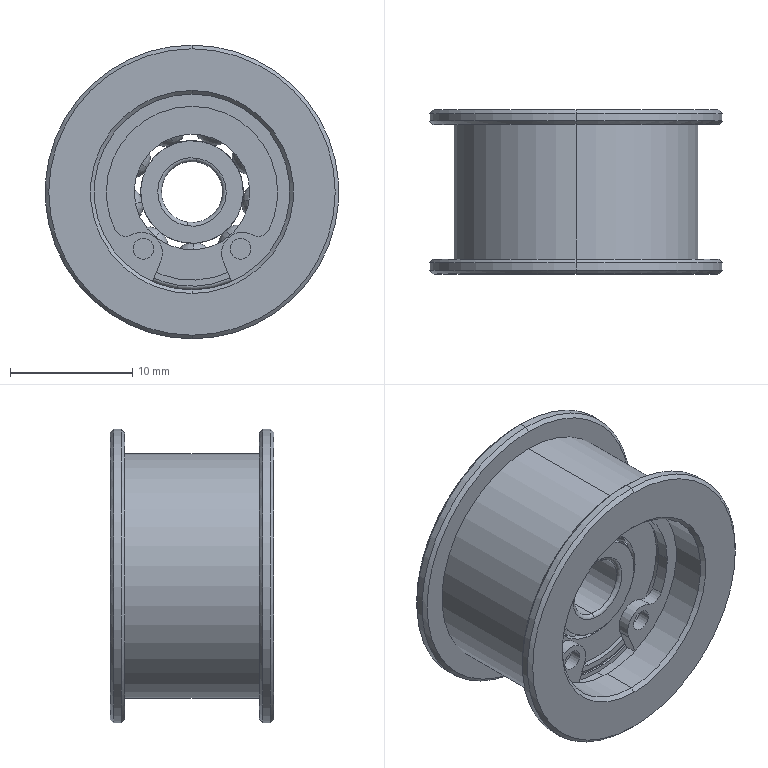Part | STEP file | Flange idler ENG11-D20-T11 | 3 solids | 212 faces | box 24 x 13.4 x 24 mm | volume 3034 mm3 | sphere 72 | cylinder 53 | torus 38 | plane 37 | cone 12 | commonest cylinder face diameters 14.4 x8 16 x6 1.7 x4 8.4 x4 9.456 x4 24 x4